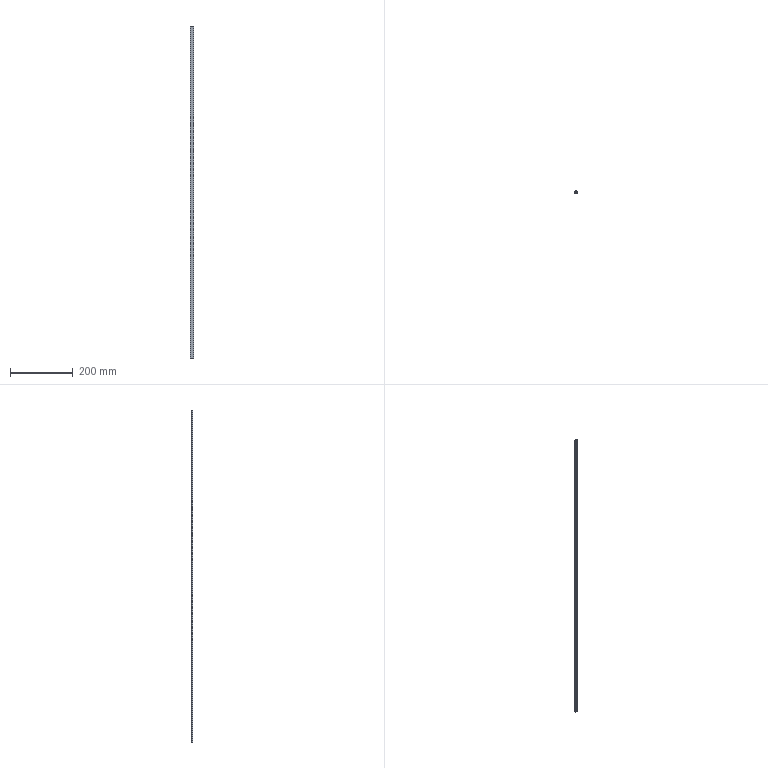Part | SolidWorks | features Extrusion 1 | 1 solid | 20 faces | box 10 x 6 x 1058 mm | volume 14916 mm3 | plane 12 | cylinder 8 | commonest cylinder face diameters 1 x3 2 x3 11.891 x1 12.891 x1
STEP:
#1=CARTESIAN_POINT('',(-4.13,5.131,529.));
#2=VERTEX_POINT('',#1);
#3=CARTESIAN_POINT('',(-4.283,4.771,529.));
#4=VERTEX_POINT('',#3);
#5=CARTESIAN_POINT('',(-3.783,4.771,529.));
#6=DIRECTION('',(0.,0.,1.));
#7=DIRECTION('',(1.,0.,0.));
#8=AXIS2_PLACEMENT_3D('',#5,#6,#7);
#9=CIRCLE('',#8,0.5);
#10=EDGE_CURVE('',#2,#4,#9,.T.);
#11=ORIENTED_EDGE('',*,*,#10,.T.);
#12=CARTESIAN_POINT('',(-4.283,4.771,-529.));
#13=VERTEX_POINT('',#12);
#14=CARTESIAN_POINT('',(-4.283,4.771,529.));
#15=DIRECTION('',(0.,0.,-1.));
#16=VECTOR('',#15,1000.);
#17=LINE('',#14,#16);
#18=EDGE_CURVE('',#4,#13,#17,.T.);
#19=ORIENTED_EDGE('',*,*,#18,.T.);
#20=CARTESIAN_POINT('',(-4.13,5.131,-529.));
#21=VERTEX_POINT('',#20);
#22=CARTESIAN_POINT('',(-3.783,4.771,-529.));
#23=DIRECTION('',(0.,0.,1.));
#24=DIRECTION('',(1.,0.,0.));
#25=AXIS2_PLACEMENT_3D('',#22,#23,#24);
#26=CIRCLE('',#25,0.5);
#27=EDGE_CURVE('',#21,#13,#26,.T.);
#28=ORIENTED_EDGE('',*,*,#27,.F.);
#29=CARTESIAN_POINT('',(-4.13,5.131,529.));
#30=DIRECTION('',(0.,0.,-1.));
#31=VECTOR('',#30,1000.);
#32=LINE('',#29,#31);
#33=EDGE_CURVE('',#2,#21,#32,.T.);
#34=ORIENTED_EDGE('',*,*,#33,.F.);
#35=EDGE_LOOP('',(#11,#19,#28,#34));
#36=FACE_OUTER_BOUND('',#35,.T.);
#37=CARTESIAN_POINT('',(-3.783,4.771,529.));
#38=DIRECTION('',(0.,0.,-1.));
#39=DIRECTION('',(-1.,0.,0.));
#40=AXIS2_PLACEMENT_3D('',#37,#38,#39);
#41=CYLINDRICAL_SURFACE('',#40,0.5);
#42=ADVANCED_FACE('',(#36),#41,.F.);
#43=CARTESIAN_POINT('',(-4.783,4.771,529.));
#44=VERTEX_POINT('',#43);
#45=CARTESIAN_POINT('',(-4.557,4.138,529.));
#46=VERTEX_POINT('',#45);
#47=CARTESIAN_POINT('',(-3.783,4.771,529.));
#48=DIRECTION('',(0.,0.,1.));
#49=DIRECTION('',(1.,0.,0.));
#50=AXIS2_PLACEMENT_3D('',#47,#48,#49);
#51=CIRCLE('',#50,1.);
#52=EDGE_CURVE('',#44,#46,#51,.T.);
#53=ORIENTED_EDGE('',*,*,#52,.F.);
#54=CARTESIAN_POINT('',(-4.783,4.771,-529.));
#55=VERTEX_POINT('',#54);
#56=CARTESIAN_POINT('',(-4.783,4.771,529.));
#57=DIRECTION('',(0.,0.,-1.));
#58=VECTOR('',#57,1000.);
#59=LINE('',#56,#58);
#60=EDGE_CURVE('',#44,#55,#59,.T.);
#61=ORIENTED_EDGE('',*,*,#60,.T.);
#62=CARTESIAN_POINT('',(-4.557,4.138,-529.));
#63=VERTEX_POINT('',#62);
#64=CARTESIAN_POINT('',(-3.783,4.771,-529.));
#65=DIRECTION('',(0.,0.,1.));
#66=DIRECTION('',(1.,0.,0.));
#67=AXIS2_PLACEMENT_3D('',#64,#65,#66);
#68=CIRCLE('',#67,1.);
#69=EDGE_CURVE('',#55,#63,#68,.T.);
#70=ORIENTED_EDGE('',*,*,#69,.T.);
#71=CARTESIAN_POINT('',(-4.557,4.138,529.));
#72=DIRECTION('',(0.,0.,-1.));
#73=VECTOR('',#72,1000.);
#74=LINE('',#71,#73);
#75=EDGE_CURVE('',#46,#63,#74,.T.);
#76=ORIENTED_EDGE('',*,*,#75,.F.);
#77=EDGE_LOOP('',(#53,#61,#70,#76));
#78=FACE_OUTER_BOUND('',#77,.T.);
#79=CARTESIAN_POINT('',(-3.783,4.771,529.));
#80=DIRECTION('',(0.,0.,-1.));
#81=DIRECTION('',(-1.,0.,0.));
#82=AXIS2_PLACEMENT_3D('',#79,#80,#81);
#83=CYLINDRICAL_SURFACE('',#82,1.);
#84=ADVANCED_FACE('',(#78),#83,.T.);
#85=CARTESIAN_POINT('',(-2.646,1.799,529.));
#86=VERTEX_POINT('',#85);
#87=CARTESIAN_POINT('',(-5.,1.799,529.));
#88=VERTEX_POINT('',#87);
#89=CARTESIAN_POINT('',(-2.646,1.799,529.));
#90=DIRECTION('',(-1.,0.,0.));
#91=VECTOR('',#90,1000.);
#92=LINE('',#89,#91);
#93=EDGE_CURVE('',#86,#88,#92,.T.);
#94=ORIENTED_EDGE('',*,*,#93,.T.);
#95=CARTESIAN_POINT('',(-5.,1.299,529.));
#96=VERTEX_POINT('',#95);
#97=CARTESIAN_POINT('',(-5.,1.799,529.));
#98=DIRECTION('',(0.,-1.,0.));
#99=VECTOR('',#98,1000.);
#100=LINE('',#97,#99);
#101=EDGE_CURVE('',#88,#96,#100,.T.);
#102=ORIENTED_EDGE('',*,*,#101,.T.);
#103=CARTESIAN_POINT('',(5.,1.299,529.));
#104=VERTEX_POINT('',#103);
#105=CARTESIAN_POINT('',(1.591,1.299,529.));
#106=DIRECTION('',(1.,0.,0.));
#107=VECTOR('',#106,1000.);
#108=LINE('',#105,#107);
#109=EDGE_CURVE('',#96,#104,#108,.T.);
#110=ORIENTED_EDGE('',*,*,#109,.T.);
#111=CARTESIAN_POINT('',(5.,1.799,529.));
#112=VERTEX_POINT('',#111);
#113=CARTESIAN_POINT('',(5.,1.799,529.));
#114=DIRECTION('',(0.,1.,0.));
#115=VECTOR('',#114,1000.);
#116=LINE('',#113,#115);
#117=EDGE_CURVE('',#104,#112,#116,.T.);
#118=ORIENTED_EDGE('',*,*,#117,.T.);
#119=CARTESIAN_POINT('',(2.646,1.799,529.));
#120=VERTEX_POINT('',#119);
#121=CARTESIAN_POINT('',(2.646,1.799,529.));
#122=DIRECTION('',(-1.,0.,0.));
#123=VECTOR('',#122,1000.);
#124=LINE('',#121,#123);
#125=EDGE_CURVE('',#112,#120,#124,.T.);
#126=ORIENTED_EDGE('',*,*,#125,.T.);
#127=CARTESIAN_POINT('',(4.557,4.138,529.));
#128=VERTEX_POINT('',#127);
#129=CARTESIAN_POINT('',(4.557,4.138,529.));
#130=DIRECTION('',(0.6327,0.7744,0.));
#131=VECTOR('',#130,1000.);
#132=LINE('',#129,#131);
#133=EDGE_CURVE('',#120,#128,#132,.T.);
#134=ORIENTED_EDGE('',*,*,#133,.T.);
#135=CARTESIAN_POINT('',(4.477,5.49,529.));
#136=VERTEX_POINT('',#135);
#137=CARTESIAN_POINT('',(3.783,4.771,529.));
#138=DIRECTION('',(0.,0.,1.));
#139=DIRECTION('',(-1.,0.,0.));
#140=AXIS2_PLACEMENT_3D('',#137,#138,#139);
#141=CIRCLE('',#140,1.);
#142=EDGE_CURVE('',#128,#136,#141,.T.);
#143=ORIENTED_EDGE('',*,*,#142,.T.);
#144=CARTESIAN_POINT('',(-4.477,5.49,529.));
#145=VERTEX_POINT('',#144);
#146=CARTESIAN_POINT('',(0.,0.8534,529.));
#147=DIRECTION('',(0.,0.,1.));
#148=DIRECTION('',(-1.,0.,0.));
#149=AXIS2_PLACEMENT_3D('',#146,#147,#148);
#150=CIRCLE('',#149,6.446);
#151=EDGE_CURVE('',#136,#145,#150,.T.);
#152=ORIENTED_EDGE('',*,*,#151,.T.);
#153=CARTESIAN_POINT('',(-3.783,4.771,529.));
#154=DIRECTION('',(0.,0.,1.));
#155=DIRECTION('',(1.,0.,0.));
#156=AXIS2_PLACEMENT_3D('',#153,#154,#155);
#157=CIRCLE('',#156,1.);
#158=EDGE_CURVE('',#145,#44,#157,.T.);
#159=ORIENTED_EDGE('',*,*,#158,.T.);
#160=ORIENTED_EDGE('',*,*,#52,.T.);
#161=CARTESIAN_POINT('',(-4.557,4.138,529.));
#162=DIRECTION('',(0.6327,-0.7744,0.));
#163=VECTOR('',#162,1000.);
#164=LINE('',#161,#163);
#165=EDGE_CURVE('',#46,#86,#164,.T.);
#166=ORIENTED_EDGE('',*,*,#165,.T.);
#167=EDGE_LOOP('',(#94,#102,#110,#118,#126,#134,#143,#152,#159,#160,#166));
#168=FACE_OUTER_BOUND('',#167,.T.);
#169=ORIENTED_EDGE('',*,*,#10,.F.);
#170=CARTESIAN_POINT('',(4.13,5.131,529.));
#171=VERTEX_POINT('',#170);
#172=CARTESIAN_POINT('',(0.,0.8534,529.));
#173=DIRECTION('',(0.,0.,1.));
#174=DIRECTION('',(-1.,0.,0.));
#175=AXIS2_PLACEMENT_3D('',#172,#173,#174);
#176=CIRCLE('',#175,5.946);
#177=EDGE_CURVE('',#171,#2,#176,.T.);
#178=ORIENTED_EDGE('',*,*,#177,.F.);
#179=CARTESIAN_POINT('',(4.17,4.454,529.));
#180=VERTEX_POINT('',#179);
#181=CARTESIAN_POINT('',(3.783,4.771,529.));
#182=DIRECTION('',(0.,0.,1.));
#183=DIRECTION('',(-1.,0.,0.));
#184=AXIS2_PLACEMENT_3D('',#181,#182,#183);
#185=CIRCLE('',#184,0.5);
#186=EDGE_CURVE('',#180,#171,#185,.T.);
#187=ORIENTED_EDGE('',*,*,#186,.F.);
#188=CARTESIAN_POINT('',(2.,1.799,529.));
#189=VERTEX_POINT('',#188);
#190=CARTESIAN_POINT('',(4.17,4.454,529.));
#191=DIRECTION('',(0.6327,0.7744,0.));
#192=VECTOR('',#191,1000.);
#193=LINE('',#190,#192);
#194=EDGE_CURVE('',#189,#180,#193,.T.);
#195=ORIENTED_EDGE('',*,*,#194,.F.);
#196=CARTESIAN_POINT('',(-2.,1.799,529.));
#197=VERTEX_POINT('',#196);
#198=CARTESIAN_POINT('',(-2.,1.799,529.));
#199=DIRECTION('',(1.,0.,0.));
#200=VECTOR('',#199,1000.);
#201=LINE('',#198,#200);
#202=EDGE_CURVE('',#197,#189,#201,.T.);
#203=ORIENTED_EDGE('',*,*,#202,.F.);
#204=CARTESIAN_POINT('',(-4.17,4.454,529.));
#205=VERTEX_POINT('',#204);
#206=CARTESIAN_POINT('',(-4.17,4.454,529.));
#207=DIRECTION('',(0.6327,-0.7744,0.));
#208=VECTOR('',#207,1000.);
#209=LINE('',#206,#208);
#210=EDGE_CURVE('',#205,#197,#209,.T.);
#211=ORIENTED_EDGE('',*,*,#210,.F.);
#212=CARTESIAN_POINT('',(-3.783,4.771,529.));
#213=DIRECTION('',(0.,0.,1.));
#214=DIRECTION('',(1.,0.,0.));
#215=AXIS2_PLACEMENT_3D('',#212,#213,#214);
#216=CIRCLE('',#215,0.5);
#217=EDGE_CURVE('',#4,#205,#216,.T.);
#218=ORIENTED_EDGE('',*,*,#217,.F.);
#219=EDGE_LOOP('',(#169,#178,#187,#195,#203,#211,#218));
#220=FACE_BOUND('',#219,.T.);
#221=CARTESIAN_POINT('',(3.783,4.771,529.));
#222=DIRECTION('',(0.,0.,-1.));
#223=DIRECTION('',(-1.,0.,0.));
#224=AXIS2_PLACEMENT_3D('',#221,#222,#223);
#225=PLANE('',#224);
#226=ADVANCED_FACE('',(#168,#220),#225,.F.);
#227=CARTESIAN_POINT('',(-2.646,1.799,-529.));
#228=VERTEX_POINT('',#227);
#229=CARTESIAN_POINT('',(-5.,1.799,-529.));
#230=VERTEX_POINT('',#229);
#231=CARTESIAN_POINT('',(-2.646,1.799,-529.));
#232=DIRECTION('',(-1.,0.,0.));
#233=VECTOR('',#232,1000.);
#234=LINE('',#231,#233);
#235=EDGE_CURVE('',#228,#230,#234,.T.);
#236=ORIENTED_EDGE('',*,*,#235,.F.);
#237=CARTESIAN_POINT('',(-4.557,4.138,-529.));
#238=DIRECTION('',(0.6327,-0.7744,0.));
#239=VECTOR('',#238,1000.);
#240=LINE('',#237,#239);
#241=EDGE_CURVE('',#63,#228,#240,.T.);
#242=ORIENTED_EDGE('',*,*,#241,.F.);
#243=ORIENTED_EDGE('',*,*,#69,.F.);
#244=CARTESIAN_POINT('',(-4.477,5.49,-529.));
#245=VERTEX_POINT('',#244);
#246=CARTESIAN_POINT('',(-3.783,4.771,-529.));
#247=DIRECTION('',(0.,0.,1.));
#248=DIRECTION('',(1.,0.,0.));
#249=AXIS2_PLACEMENT_3D('',#246,#247,#248);
#250=CIRCLE('',#249,1.);
#251=EDGE_CURVE('',#245,#55,#250,.T.);
#252=ORIENTED_EDGE('',*,*,#251,.F.);
#253=CARTESIAN_POINT('',(4.477,5.49,-529.));
#254=VERTEX_POINT('',#253);
#255=CARTESIAN_POINT('',(0.,0.8534,-529.));
#256=DIRECTION('',(0.,0.,1.));
#257=DIRECTION('',(-1.,0.,0.));
#258=AXIS2_PLACEMENT_3D('',#255,#256,#257);
#259=CIRCLE('',#258,6.446);
#260=EDGE_CURVE('',#254,#245,#259,.T.);
#261=ORIENTED_EDGE('',*,*,#260,.F.);
#262=CARTESIAN_POINT('',(4.557,4.138,-529.));
#263=VERTEX_POINT('',#262);
#264=CARTESIAN_POINT('',(3.783,4.771,-529.));
#265=DIRECTION('',(0.,0.,1.));
#266=DIRECTION('',(-1.,0.,0.));
#267=AXIS2_PLACEMENT_3D('',#264,#265,#266);
#268=CIRCLE('',#267,1.);
#269=EDGE_CURVE('',#263,#254,#268,.T.);
#270=ORIENTED_EDGE('',*,*,#269,.F.);
#271=CARTESIAN_POINT('',(2.646,1.799,-529.));
#272=VERTEX_POINT('',#271);
#273=CARTESIAN_POINT('',(4.557,4.138,-529.));
#274=DIRECTION('',(0.6327,0.7744,0.));
#275=VECTOR('',#274,1000.);
#276=LINE('',#273,#275);
#277=EDGE_CURVE('',#272,#263,#276,.T.);
#278=ORIENTED_EDGE('',*,*,#277,.F.);
#279=CARTESIAN_POINT('',(5.,1.799,-529.));
#280=VERTEX_POINT('',#279);
#281=CARTESIAN_POINT('',(2.646,1.799,-529.));
#282=DIRECTION('',(-1.,0.,0.));
#283=VECTOR('',#282,1000.);
#284=LINE('',#281,#283);
#285=EDGE_CURVE('',#280,#272,#284,.T.);
#286=ORIENTED_EDGE('',*,*,#285,.F.);
#287=CARTESIAN_POINT('',(5.,1.299,-529.));
#288=VERTEX_POINT('',#287);
#289=CARTESIAN_POINT('',(5.,1.799,-529.));
#290=DIRECTION('',(0.,1.,0.));
#291=VECTOR('',#290,1000.);
#292=LINE('',#289,#291);
#293=EDGE_CURVE('',#288,#280,#292,.T.);
#294=ORIENTED_EDGE('',*,*,#293,.F.);
#295=CARTESIAN_POINT('',(-5.,1.299,-529.));
#296=VERTEX_POINT('',#295);
#297=CARTESIAN_POINT('',(1.591,1.299,-529.));
#298=DIRECTION('',(1.,0.,0.));
#299=VECTOR('',#298,1000.);
#300=LINE('',#297,#299);
#301=EDGE_CURVE('',#296,#288,#300,.T.);
#302=ORIENTED_EDGE('',*,*,#301,.F.);
#303=CARTESIAN_POINT('',(-5.,1.799,-529.));
#304=DIRECTION('',(0.,-1.,0.));
#305=VECTOR('',#304,1000.);
#306=LINE('',#303,#305);
#307=EDGE_CURVE('',#230,#296,#306,.T.);
#308=ORIENTED_EDGE('',*,*,#307,.F.);
#309=EDGE_LOOP('',(#236,#242,#243,#252,#261,#270,#278,#286,#294,#302,#308));
#310=FACE_OUTER_BOUND('',#309,.T.);
#311=CARTESIAN_POINT('',(4.13,5.131,-529.));
#312=VERTEX_POINT('',#311);
#313=CARTESIAN_POINT('',(0.,0.8534,-529.));
#314=DIRECTION('',(0.,0.,1.));
#315=DIRECTION('',(-1.,0.,0.));
#316=AXIS2_PLACEMENT_3D('',#313,#314,#315);
#317=CIRCLE('',#316,5.946);
#318=EDGE_CURVE('',#312,#21,#317,.T.);
#319=ORIENTED_EDGE('',*,*,#318,.T.);
#320=ORIENTED_EDGE('',*,*,#27,.T.);
#321=CARTESIAN_POINT('',(-4.17,4.454,-529.));
#322=VERTEX_POINT('',#321);
#323=CARTESIAN_POINT('',(-3.783,4.771,-529.));
#324=DIRECTION('',(0.,0.,1.));
#325=DIRECTION('',(1.,0.,0.));
#326=AXIS2_PLACEMENT_3D('',#323,#324,#325);
#327=CIRCLE('',#326,0.5);
#328=EDGE_CURVE('',#13,#322,#327,.T.);
#329=ORIENTED_EDGE('',*,*,#328,.T.);
#330=CARTESIAN_POINT('',(-2.,1.799,-529.));
#331=VERTEX_POINT('',#330);
#332=CARTESIAN_POINT('',(-4.17,4.454,-529.));
#333=DIRECTION('',(0.6327,-0.7744,0.));
#334=VECTOR('',#333,1000.);
#335=LINE('',#332,#334);
#336=EDGE_CURVE('',#322,#331,#335,.T.);
#337=ORIENTED_EDGE('',*,*,#336,.T.);
#338=CARTESIAN_POINT('',(2.,1.799,-529.));
#339=VERTEX_POINT('',#338);
#340=CARTESIAN_POINT('',(-2.,1.799,-529.));
#341=DIRECTION('',(1.,0.,0.));
#342=VECTOR('',#341,1000.);
#343=LINE('',#340,#342);
#344=EDGE_CURVE('',#331,#339,#343,.T.);
#345=ORIENTED_EDGE('',*,*,#344,.T.);
#346=CARTESIAN_POINT('',(4.17,4.454,-529.));
#347=VERTEX_POINT('',#346);
#348=CARTESIAN_POINT('',(4.17,4.454,-529.));
#349=DIRECTION('',(0.6327,0.7744,0.));
#350=VECTOR('',#349,1000.);
#351=LINE('',#348,#350);
#352=EDGE_CURVE('',#339,#347,#351,.T.);
#353=ORIENTED_EDGE('',*,*,#352,.T.);
#354=CARTESIAN_POINT('',(3.783,4.771,-529.));
#355=DIRECTION('',(0.,0.,1.));
#356=DIRECTION('',(-1.,0.,0.));
#357=AXIS2_PLACEMENT_3D('',#354,#355,#356);
#358=CIRCLE('',#357,0.5);
#359=EDGE_CURVE('',#347,#312,#358,.T.);
#360=ORIENTED_EDGE('',*,*,#359,.T.);
#361=EDGE_LOOP('',(#319,#320,#329,#337,#345,#353,#360));
#362=FACE_BOUND('',#361,.T.);
#363=CARTESIAN_POINT('',(3.783,4.771,-529.));
#364=DIRECTION('',(0.,0.,-1.));
#365=DIRECTION('',(-1.,0.,0.));
#366=AXIS2_PLACEMENT_3D('',#363,#364,#365);
#367=PLANE('',#366);
#368=ADVANCED_FACE('',(#310,#362),#367,.T.);
#369=ORIENTED_EDGE('',*,*,#235,.T.);
#370=CARTESIAN_POINT('',(-5.,1.799,529.));
#371=DIRECTION('',(0.,0.,-1.));
#372=VECTOR('',#371,1000.);
#373=LINE('',#370,#372);
#374=EDGE_CURVE('',#88,#230,#373,.T.);
#375=ORIENTED_EDGE('',*,*,#374,.F.);
#376=ORIENTED_EDGE('',*,*,#93,.F.);
#377=CARTESIAN_POINT('',(-2.646,1.799,529.));
#378=DIRECTION('',(0.,0.,-1.));
#379=VECTOR('',#378,1000.);
#380=LINE('',#377,#379);
#381=EDGE_CURVE('',#86,#228,#380,.T.);
#382=ORIENTED_EDGE('',*,*,#381,.T.);
#383=EDGE_LOOP('',(#369,#375,#376,#382));
#384=FACE_OUTER_BOUND('',#383,.T.);
#385=CARTESIAN_POINT('',(-2.646,1.799,529.));
#386=DIRECTION('',(0.,-1.,0.));
#387=DIRECTION('',(1.,0.,0.));
#388=AXIS2_PLACEMENT_3D('',#385,#386,#387);
#389=PLANE('',#388);
#390=ADVANCED_FACE('',(#384),#389,.F.);
#391=ORIENTED_EDGE('',*,*,#307,.T.);
#392=CARTESIAN_POINT('',(-5.,1.299,529.));
#393=DIRECTION('',(0.,0.,-1.));
#394=VECTOR('',#393,1000.);
#395=LINE('',#392,#394);
#396=EDGE_CURVE('',#96,#296,#395,.T.);
#397=ORIENTED_EDGE('',*,*,#396,.F.);
#398=ORIENTED_EDGE('',*,*,#101,.F.);
#399=ORIENTED_EDGE('',*,*,#374,.T.);
#400=EDGE_LOOP('',(#391,#397,#398,#399));
#401=FACE_OUTER_BOUND('',#400,.T.);
#402=CARTESIAN_POINT('',(-5.,1.799,529.));
#403=DIRECTION('',(1.,0.,0.));
#404=DIRECTION('',(0.,0.,-1.));
#405=AXIS2_PLACEMENT_3D('',#402,#403,#404);
#406=PLANE('',#405);
#407=ADVANCED_FACE('',(#401),#406,.F.);
#408=ORIENTED_EDGE('',*,*,#301,.T.);
#409=CARTESIAN_POINT('',(5.,1.299,529.));
#410=DIRECTION('',(0.,0.,-1.));
#411=VECTOR('',#410,1000.);
#412=LINE('',#409,#411);
#413=EDGE_CURVE('',#104,#288,#412,.T.);
#414=ORIENTED_EDGE('',*,*,#413,.F.);
#415=ORIENTED_EDGE('',*,*,#109,.F.);
#416=ORIENTED_EDGE('',*,*,#396,.T.);
#417=EDGE_LOOP('',(#408,#414,#415,#416));
#418=FACE_OUTER_BOUND('',#417,.T.);
#419=CARTESIAN_POINT('',(1.591,1.299,529.));
#420=DIRECTION('',(0.,1.,0.));
#421=DIRECTION('',(-1.,0.,0.));
#422=AXIS2_PLACEMENT_3D('',#419,#420,#421);
#423=PLANE('',#422);
#424=ADVANCED_FACE('',(#418),#423,.F.);
#425=ORIENTED_EDGE('',*,*,#293,.T.);
#426=CARTESIAN_POINT('',(5.,1.799,529.));
#427=DIRECTION('',(0.,0.,-1.));
#428=VECTOR('',#427,1000.);
#429=LINE('',#426,#428);
#430=EDGE_CURVE('',#112,#280,#429,.T.);
#431=ORIENTED_EDGE('',*,*,#430,.F.);
#432=ORIENTED_EDGE('',*,*,#117,.F.);
#433=ORIENTED_EDGE('',*,*,#413,.T.);
#434=EDGE_LOOP('',(#425,#431,#432,#433));
#435=FACE_OUTER_BOUND('',#434,.T.);
#436=CARTESIAN_POINT('',(5.,1.799,529.));
#437=DIRECTION('',(-1.,0.,0.));
#438=DIRECTION('',(0.,0.,1.));
#439=AXIS2_PLACEMENT_3D('',#436,#437,#438);
#440=PLANE('',#439);
#441=ADVANCED_FACE('',(#435),#440,.F.);
#442=ORIENTED_EDGE('',*,*,#285,.T.);
#443=CARTESIAN_POINT('',(2.646,1.799,529.));
#444=DIRECTION('',(0.,0.,-1.));
#445=VECTOR('',#444,1000.);
#446=LINE('',#443,#445);
#447=EDGE_CURVE('',#120,#272,#446,.T.);
#448=ORIENTED_EDGE('',*,*,#447,.F.);
#449=ORIENTED_EDGE('',*,*,#125,.F.);
#450=ORIENTED_EDGE('',*,*,#430,.T.);
#451=EDGE_LOOP('',(#442,#448,#449,#450));
#452=FACE_OUTER_BOUND('',#451,.T.);
#453=CARTESIAN_POINT('',(2.646,1.799,529.));
#454=DIRECTION('',(0.,-1.,0.));
#455=DIRECTION('',(1.,0.,0.));
#456=AXIS2_PLACEMENT_3D('',#453,#454,#455);
#457=PLANE('',#456);
#458=ADVANCED_FACE('',(#452),#457,.F.);
#459=ORIENTED_EDGE('',*,*,#277,.T.);
#460=CARTESIAN_POINT('',(4.557,4.138,529.));
#461=DIRECTION('',(0.,0.,-1.));
#462=VECTOR('',#461,1000.);
#463=LINE('',#460,#462);
#464=EDGE_CURVE('',#128,#263,#463,.T.);
#465=ORIENTED_EDGE('',*,*,#464,.F.);
#466=ORIENTED_EDGE('',*,*,#133,.F.);
#467=ORIENTED_EDGE('',*,*,#447,.T.);
#468=EDGE_LOOP('',(#459,#465,#466,#467));
#469=FACE_OUTER_BOUND('',#468,.T.);
#470=CARTESIAN_POINT('',(4.557,4.138,529.));
#471=DIRECTION('',(-0.7744,0.6327,0.));
#472=DIRECTION('',(-0.6327,-0.7744,0.));
#473=AXIS2_PLACEMENT_3D('',#470,#471,#472);
#474=PLANE('',#473);
#475=ADVANCED_FACE('',(#469),#474,.F.);
#476=ORIENTED_EDGE('',*,*,#269,.T.);
#477=CARTESIAN_POINT('',(4.477,5.49,529.));
#478=DIRECTION('',(0.,0.,-1.));
#479=VECTOR('',#478,1000.);
#480=LINE('',#477,#479);
#481=EDGE_CURVE('',#136,#254,#480,.T.);
#482=ORIENTED_EDGE('',*,*,#481,.F.);
#483=ORIENTED_EDGE('',*,*,#142,.F.);
#484=ORIENTED_EDGE('',*,*,#464,.T.);
#485=EDGE_LOOP('',(#476,#482,#483,#484));
#486=FACE_OUTER_BOUND('',#485,.T.);
#487=CARTESIAN_POINT('',(3.783,4.771,529.));
#488=DIRECTION('',(0.,0.,-1.));
#489=DIRECTION('',(-1.,0.,0.));
#490=AXIS2_PLACEMENT_3D('',#487,#488,#489);
#491=CYLINDRICAL_SURFACE('',#490,1.);
#492=ADVANCED_FACE('',(#486),#491,.T.);
#493=ORIENTED_EDGE('',*,*,#260,.T.);
#494=CARTESIAN_POINT('',(-4.477,5.49,529.));
#495=DIRECTION('',(0.,0.,-1.));
#496=VECTOR('',#495,1000.);
#497=LINE('',#494,#496);
#498=EDGE_CURVE('',#145,#245,#497,.T.);
#499=ORIENTED_EDGE('',*,*,#498,.F.);
#500=ORIENTED_EDGE('',*,*,#151,.F.);
#501=ORIENTED_EDGE('',*,*,#481,.T.);
#502=EDGE_LOOP('',(#493,#499,#500,#501));
#503=FACE_OUTER_BOUND('',#502,.T.);
#504=CARTESIAN_POINT('',(0.,0.8534,529.));
#505=DIRECTION('',(0.,0.,-1.));
#506=DIRECTION('',(-1.,0.,0.));
#507=AXIS2_PLACEMENT_3D('',#504,#505,#506);
#508=CYLINDRICAL_SURFACE('',#507,6.446);
#509=ADVANCED_FACE('',(#503),#508,.T.);
#510=ORIENTED_EDGE('',*,*,#60,.F.);
#511=ORIENTED_EDGE('',*,*,#158,.F.);
#512=ORIENTED_EDGE('',*,*,#498,.T.);
#513=ORIENTED_EDGE('',*,*,#251,.T.);
#514=EDGE_LOOP('',(#510,#511,#512,#513));
#515=FACE_OUTER_BOUND('',#514,.T.);
#516=CARTESIAN_POINT('',(-3.783,4.771,529.));
#517=DIRECTION('',(0.,0.,-1.));
#518=DIRECTION('',(-1.,0.,0.));
#519=AXIS2_PLACEMENT_3D('',#516,#517,#518);
#520=CYLINDRICAL_SURFACE('',#519,1.);
#521=ADVANCED_FACE('',(#515),#520,.T.);
#522=ORIENTED_EDGE('',*,*,#241,.T.);
#523=ORIENTED_EDGE('',*,*,#381,.F.);
#524=ORIENTED_EDGE('',*,*,#165,.F.);
#525=ORIENTED_EDGE('',*,*,#75,.T.);
#526=EDGE_LOOP('',(#522,#523,#524,#525));
#527=FACE_OUTER_BOUND('',#526,.T.);
#528=CARTESIAN_POINT('',(-4.557,4.138,529.));
#529=DIRECTION('',(0.7744,0.6327,0.));
#530=DIRECTION('',(-0.6327,0.7744,0.));
#531=AXIS2_PLACEMENT_3D('',#528,#529,#530);
#532=PLANE('',#531);
#533=ADVANCED_FACE('',(#527),#532,.F.);
#534=ORIENTED_EDGE('',*,*,#18,.F.);
#535=ORIENTED_EDGE('',*,*,#217,.T.);
#536=CARTESIAN_POINT('',(-4.17,4.454,529.));
#537=DIRECTION('',(0.,0.,-1.));
#538=VECTOR('',#537,1000.);
#539=LINE('',#536,#538);
#540=EDGE_CURVE('',#205,#322,#539,.T.);
#541=ORIENTED_EDGE('',*,*,#540,.T.);
#542=ORIENTED_EDGE('',*,*,#328,.F.);
#543=EDGE_LOOP('',(#534,#535,#541,#542));
#544=FACE_OUTER_BOUND('',#543,.T.);
#545=CARTESIAN_POINT('',(-3.783,4.771,529.));
#546=DIRECTION('',(0.,0.,-1.));
#547=DIRECTION('',(-1.,0.,0.));
#548=AXIS2_PLACEMENT_3D('',#545,#546,#547);
#549=CYLINDRICAL_SURFACE('',#548,0.5);
#550=ADVANCED_FACE('',(#544),#549,.F.);
#551=ORIENTED_EDGE('',*,*,#336,.F.);
#552=ORIENTED_EDGE('',*,*,#540,.F.);
#553=ORIENTED_EDGE('',*,*,#210,.T.);
#554=CARTESIAN_POINT('',(-2.,1.799,529.));
#555=DIRECTION('',(0.,0.,-1.));
#556=VECTOR('',#555,1000.);
#557=LINE('',#554,#556);
#558=EDGE_CURVE('',#197,#331,#557,.T.);
#559=ORIENTED_EDGE('',*,*,#558,.T.);
#560=EDGE_LOOP('',(#551,#552,#553,#559));
#561=FACE_OUTER_BOUND('',#560,.T.);
#562=CARTESIAN_POINT('',(-4.17,4.454,529.));
#563=DIRECTION('',(0.7744,0.6327,0.));
#564=DIRECTION('',(-0.6327,0.7744,0.));
#565=AXIS2_PLACEMENT_3D('',#562,#563,#564);
#566=PLANE('',#565);
#567=ADVANCED_FACE('',(#561),#566,.T.);
#568=ORIENTED_EDGE('',*,*,#344,.F.);
#569=ORIENTED_EDGE('',*,*,#558,.F.);
#570=ORIENTED_EDGE('',*,*,#202,.T.);
#571=CARTESIAN_POINT('',(2.,1.799,529.));
#572=DIRECTION('',(0.,0.,-1.));
#573=VECTOR('',#572,1000.);
#574=LINE('',#571,#573);
#575=EDGE_CURVE('',#189,#339,#574,.T.);
#576=ORIENTED_EDGE('',*,*,#575,.T.);
#577=EDGE_LOOP('',(#568,#569,#570,#576));
#578=FACE_OUTER_BOUND('',#577,.T.);
#579=CARTESIAN_POINT('',(-2.,1.799,529.));
#580=DIRECTION('',(0.,1.,0.));
#581=DIRECTION('',(0.,0.,1.));
#582=AXIS2_PLACEMENT_3D('',#579,#580,#581);
#583=PLANE('',#582);
#584=ADVANCED_FACE('',(#578),#583,.T.);
#585=ORIENTED_EDGE('',*,*,#352,.F.);
#586=ORIENTED_EDGE('',*,*,#575,.F.);
#587=ORIENTED_EDGE('',*,*,#194,.T.);
#588=CARTESIAN_POINT('',(4.17,4.454,529.));
#589=DIRECTION('',(0.,0.,-1.));
#590=VECTOR('',#589,1000.);
#591=LINE('',#588,#590);
#592=EDGE_CURVE('',#180,#347,#591,.T.);
#593=ORIENTED_EDGE('',*,*,#592,.T.);
#594=EDGE_LOOP('',(#585,#586,#587,#593));
#595=FACE_OUTER_BOUND('',#594,.T.);
#596=CARTESIAN_POINT('',(4.17,4.454,529.));
#597=DIRECTION('',(-0.7744,0.6327,0.));
#598=DIRECTION('',(-0.6327,-0.7744,0.));
#599=AXIS2_PLACEMENT_3D('',#596,#597,#598);
#600=PLANE('',#599);
#601=ADVANCED_FACE('',(#595),#600,.T.);
#602=ORIENTED_EDGE('',*,*,#359,.F.);
#603=ORIENTED_EDGE('',*,*,#592,.F.);
#604=ORIENTED_EDGE('',*,*,#186,.T.);
#605=CARTESIAN_POINT('',(4.13,5.131,529.));
#606=DIRECTION('',(0.,0.,-1.));
#607=VECTOR('',#606,1000.);
#608=LINE('',#605,#607);
#609=EDGE_CURVE('',#171,#312,#608,.T.);
#610=ORIENTED_EDGE('',*,*,#609,.T.);
#611=EDGE_LOOP('',(#602,#603,#604,#610));
#612=FACE_OUTER_BOUND('',#611,.T.);
#613=CARTESIAN_POINT('',(3.783,4.771,529.));
#614=DIRECTION('',(0.,0.,-1.));
#615=DIRECTION('',(-1.,0.,0.));
#616=AXIS2_PLACEMENT_3D('',#613,#614,#615);
#617=CYLINDRICAL_SURFACE('',#616,0.5);
#618=ADVANCED_FACE('',(#612),#617,.F.);
#619=ORIENTED_EDGE('',*,*,#318,.F.);
#620=ORIENTED_EDGE('',*,*,#609,.F.);
#621=ORIENTED_EDGE('',*,*,#177,.T.);
#622=ORIENTED_EDGE('',*,*,#33,.T.);
#623=EDGE_LOOP('',(#619,#620,#621,#622));
#624=FACE_OUTER_BOUND('',#623,.T.);
#625=CARTESIAN_POINT('',(0.,0.8534,529.));
#626=DIRECTION('',(0.,0.,-1.));
#627=DIRECTION('',(-1.,0.,0.));
#628=AXIS2_PLACEMENT_3D('',#625,#626,#627);
#629=CYLINDRICAL_SURFACE('',#628,5.946);
#630=ADVANCED_FACE('',(#624),#629,.F.);
#631=CLOSED_SHELL('',(#42,#84,#226,#368,#390,#407,#424,#441,#458,#475,#492,#509,#521,#533,#550,#567,#584,#601,#618,#630));
#632=MANIFOLD_SOLID_BREP('',#631);
#633=CARTESIAN_POINT('',(0.,0.,0.));
#634=DIRECTION('',(0.,0.,1.));
#635=DIRECTION('',(1.,0.,0.));
#636=AXIS2_PLACEMENT_3D('',#633,#634,#635);
#637=(LENGTH_UNIT()NAMED_UNIT(*)SI_UNIT(.MILLI.,.METRE.));
#638=UNCERTAINTY_MEASURE_WITH_UNIT(LENGTH_MEASURE(0.00001),#637,'','');
#639=(NAMED_UNIT(*)PLANE_ANGLE_UNIT()SI_UNIT($,.RADIAN.));
#640=(NAMED_UNIT(*)SI_UNIT($,.STERADIAN.)SOLID_ANGLE_UNIT());
#641=(GEOMETRIC_REPRESENTATION_CONTEXT(3)GLOBAL_UNCERTAINTY_ASSIGNED_CONTEXT((#638))GLOBAL_UNIT_ASSIGNED_CONTEXT((#637,#639,#640))REPRESENTATION_CONTEXT('',''));
#642=ADVANCED_BREP_SHAPE_REPRESENTATION('',(#632,#636),#641);